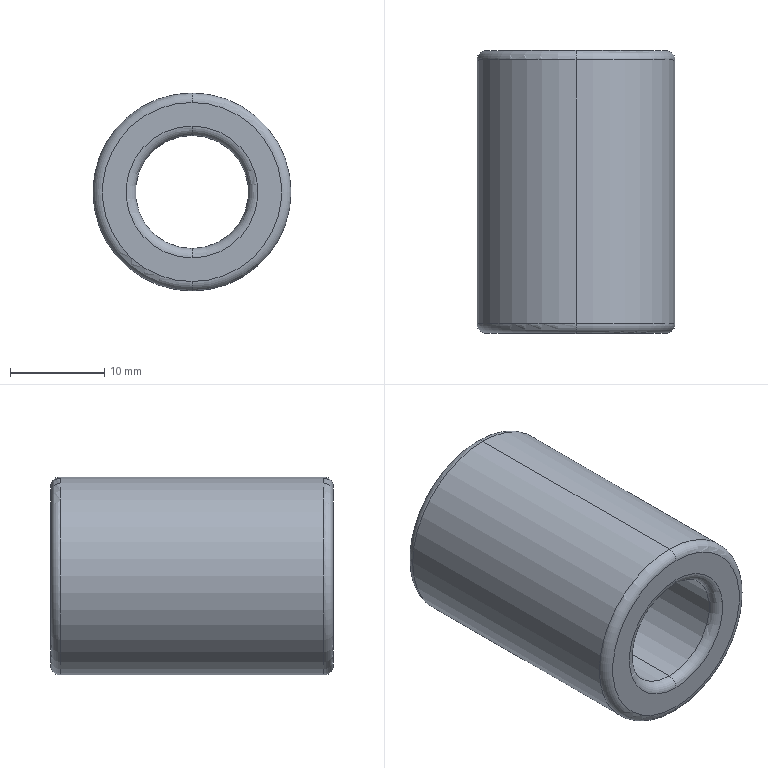Part | SolidWorks | features Extrusion 1, Fillet 1 | 1 solid | 14 faces | box 21 x 30 x 21 mm | volume 6953 mm3 | torus 8 | cylinder 4 | plane 2 | commonest cylinder face diameters 12 x2 21 x2
STEP:
#1=CARTESIAN_POINT('',(0.,29.,-10.5));
#2=VERTEX_POINT('',#1);
#3=CARTESIAN_POINT('',(0.,29.,10.5));
#4=VERTEX_POINT('',#3);
#5=CARTESIAN_POINT('',(0.,29.,0.));
#6=DIRECTION('',(0.,-1.,0.));
#7=DIRECTION('',(0.,0.,1.));
#8=AXIS2_PLACEMENT_3D('',#5,#6,#7);
#9=CIRCLE('',#8,10.5);
#10=EDGE_CURVE('',#2,#4,#9,.T.);
#11=ORIENTED_EDGE('',*,*,#10,.F.);
#12=CARTESIAN_POINT('',(0.,30.,-9.5));
#13=VERTEX_POINT('',#12);
#14=CARTESIAN_POINT('',(0.,29.,-9.5));
#15=DIRECTION('',(1.,0.,0.));
#16=DIRECTION('',(0.,0.,-1.));
#17=AXIS2_PLACEMENT_3D('',#14,#15,#16);
#18=CIRCLE('',#17,1.);
#19=EDGE_CURVE('',#2,#13,#18,.T.);
#20=ORIENTED_EDGE('',*,*,#19,.T.);
#21=CARTESIAN_POINT('',(0.,30.,9.5));
#22=VERTEX_POINT('',#21);
#23=CARTESIAN_POINT('',(0.,30.,0.));
#24=DIRECTION('',(0.,1.,0.));
#25=DIRECTION('',(0.,0.,1.));
#26=AXIS2_PLACEMENT_3D('',#23,#24,#25);
#27=CIRCLE('',#26,9.5);
#28=EDGE_CURVE('',#22,#13,#27,.T.);
#29=ORIENTED_EDGE('',*,*,#28,.F.);
#30=CARTESIAN_POINT('',(0.,29.,9.5));
#31=DIRECTION('',(-1.,0.,0.));
#32=DIRECTION('',(0.,0.,1.));
#33=AXIS2_PLACEMENT_3D('',#30,#31,#32);
#34=CIRCLE('',#33,1.);
#35=EDGE_CURVE('',#4,#22,#34,.T.);
#36=ORIENTED_EDGE('',*,*,#35,.F.);
#37=EDGE_LOOP('',(#11,#20,#29,#36));
#38=FACE_OUTER_BOUND('',#37,.T.);
#39=CARTESIAN_POINT('',(0.,29.,0.));
#40=DIRECTION('',(0.,1.,0.));
#41=DIRECTION('',(0.,0.,1.));
#42=AXIS2_PLACEMENT_3D('',#39,#40,#41);
#43=TOROIDAL_SURFACE('',#42,9.5,1.);
#44=ADVANCED_FACE('',(#38),#43,.T.);
#45=CARTESIAN_POINT('',(0.,0.,-9.5));
#46=VERTEX_POINT('',#45);
#47=CARTESIAN_POINT('',(0.,0.,9.5));
#48=VERTEX_POINT('',#47);
#49=CARTESIAN_POINT('',(0.,0.,0.));
#50=DIRECTION('',(0.,-1.,0.));
#51=DIRECTION('',(0.,0.,1.));
#52=AXIS2_PLACEMENT_3D('',#49,#50,#51);
#53=CIRCLE('',#52,9.5);
#54=EDGE_CURVE('',#46,#48,#53,.T.);
#55=ORIENTED_EDGE('',*,*,#54,.F.);
#56=CARTESIAN_POINT('',(0.,1.,-10.5));
#57=VERTEX_POINT('',#56);
#58=CARTESIAN_POINT('',(0.,1.,-9.5));
#59=DIRECTION('',(1.,0.,0.));
#60=DIRECTION('',(0.,0.,-1.));
#61=AXIS2_PLACEMENT_3D('',#58,#59,#60);
#62=CIRCLE('',#61,1.);
#63=EDGE_CURVE('',#46,#57,#62,.T.);
#64=ORIENTED_EDGE('',*,*,#63,.T.);
#65=CARTESIAN_POINT('',(0.,1.,10.5));
#66=VERTEX_POINT('',#65);
#67=CARTESIAN_POINT('',(0.,1.,0.));
#68=DIRECTION('',(0.,1.,0.));
#69=DIRECTION('',(0.,0.,1.));
#70=AXIS2_PLACEMENT_3D('',#67,#68,#69);
#71=CIRCLE('',#70,10.5);
#72=EDGE_CURVE('',#66,#57,#71,.T.);
#73=ORIENTED_EDGE('',*,*,#72,.F.);
#74=CARTESIAN_POINT('',(0.,1.,9.5));
#75=DIRECTION('',(-1.,0.,0.));
#76=DIRECTION('',(0.,0.,1.));
#77=AXIS2_PLACEMENT_3D('',#74,#75,#76);
#78=CIRCLE('',#77,1.);
#79=EDGE_CURVE('',#48,#66,#78,.T.);
#80=ORIENTED_EDGE('',*,*,#79,.F.);
#81=EDGE_LOOP('',(#55,#64,#73,#80));
#82=FACE_OUTER_BOUND('',#81,.T.);
#83=CARTESIAN_POINT('',(0.,1.,0.));
#84=DIRECTION('',(0.,1.,0.));
#85=DIRECTION('',(0.,0.,1.));
#86=AXIS2_PLACEMENT_3D('',#83,#84,#85);
#87=TOROIDAL_SURFACE('',#86,9.5,1.);
#88=ADVANCED_FACE('',(#82),#87,.T.);
#89=CARTESIAN_POINT('',(0.,30.,-7.));
#90=VERTEX_POINT('',#89);
#91=CARTESIAN_POINT('',(0.,30.,7.));
#92=VERTEX_POINT('',#91);
#93=CARTESIAN_POINT('',(0.,30.,0.));
#94=DIRECTION('',(0.,-1.,0.));
#95=DIRECTION('',(0.,0.,1.));
#96=AXIS2_PLACEMENT_3D('',#93,#94,#95);
#97=CIRCLE('',#96,7.);
#98=EDGE_CURVE('',#90,#92,#97,.T.);
#99=ORIENTED_EDGE('',*,*,#98,.F.);
#100=CARTESIAN_POINT('',(0.,29.,-6.));
#101=VERTEX_POINT('',#100);
#102=CARTESIAN_POINT('',(0.,29.,-7.));
#103=DIRECTION('',(1.,0.,0.));
#104=DIRECTION('',(0.,0.,-1.));
#105=AXIS2_PLACEMENT_3D('',#102,#103,#104);
#106=CIRCLE('',#105,1.);
#107=EDGE_CURVE('',#90,#101,#106,.T.);
#108=ORIENTED_EDGE('',*,*,#107,.T.);
#109=CARTESIAN_POINT('',(0.,29.,6.));
#110=VERTEX_POINT('',#109);
#111=CARTESIAN_POINT('',(0.,29.,0.));
#112=DIRECTION('',(0.,1.,0.));
#113=DIRECTION('',(0.,0.,1.));
#114=AXIS2_PLACEMENT_3D('',#111,#112,#113);
#115=CIRCLE('',#114,6.);
#116=EDGE_CURVE('',#110,#101,#115,.T.);
#117=ORIENTED_EDGE('',*,*,#116,.F.);
#118=CARTESIAN_POINT('',(0.,29.,7.));
#119=DIRECTION('',(-1.,0.,0.));
#120=DIRECTION('',(0.,0.,1.));
#121=AXIS2_PLACEMENT_3D('',#118,#119,#120);
#122=CIRCLE('',#121,1.);
#123=EDGE_CURVE('',#92,#110,#122,.T.);
#124=ORIENTED_EDGE('',*,*,#123,.F.);
#125=EDGE_LOOP('',(#99,#108,#117,#124));
#126=FACE_OUTER_BOUND('',#125,.T.);
#127=CARTESIAN_POINT('',(0.,29.,0.));
#128=DIRECTION('',(0.,1.,0.));
#129=DIRECTION('',(0.,0.,1.));
#130=AXIS2_PLACEMENT_3D('',#127,#128,#129);
#131=TOROIDAL_SURFACE('',#130,7.,1.);
#132=ADVANCED_FACE('',(#126),#131,.T.);
#133=CARTESIAN_POINT('',(0.,1.,-6.));
#134=VERTEX_POINT('',#133);
#135=CARTESIAN_POINT('',(0.,1.,6.));
#136=VERTEX_POINT('',#135);
#137=CARTESIAN_POINT('',(0.,1.,0.));
#138=DIRECTION('',(0.,-1.,0.));
#139=DIRECTION('',(0.,0.,1.));
#140=AXIS2_PLACEMENT_3D('',#137,#138,#139);
#141=CIRCLE('',#140,6.);
#142=EDGE_CURVE('',#134,#136,#141,.T.);
#143=ORIENTED_EDGE('',*,*,#142,.F.);
#144=CARTESIAN_POINT('',(0.,0.,-7.));
#145=VERTEX_POINT('',#144);
#146=CARTESIAN_POINT('',(0.,1.,-7.));
#147=DIRECTION('',(1.,0.,0.));
#148=DIRECTION('',(0.,0.,-1.));
#149=AXIS2_PLACEMENT_3D('',#146,#147,#148);
#150=CIRCLE('',#149,1.);
#151=EDGE_CURVE('',#134,#145,#150,.T.);
#152=ORIENTED_EDGE('',*,*,#151,.T.);
#153=CARTESIAN_POINT('',(0.,0.,7.));
#154=VERTEX_POINT('',#153);
#155=CARTESIAN_POINT('',(0.,0.,0.));
#156=DIRECTION('',(0.,1.,0.));
#157=DIRECTION('',(0.,0.,1.));
#158=AXIS2_PLACEMENT_3D('',#155,#156,#157);
#159=CIRCLE('',#158,7.);
#160=EDGE_CURVE('',#154,#145,#159,.T.);
#161=ORIENTED_EDGE('',*,*,#160,.F.);
#162=CARTESIAN_POINT('',(0.,1.,7.));
#163=DIRECTION('',(-1.,0.,0.));
#164=DIRECTION('',(0.,0.,1.));
#165=AXIS2_PLACEMENT_3D('',#162,#163,#164);
#166=CIRCLE('',#165,1.);
#167=EDGE_CURVE('',#136,#154,#166,.T.);
#168=ORIENTED_EDGE('',*,*,#167,.F.);
#169=EDGE_LOOP('',(#143,#152,#161,#168));
#170=FACE_OUTER_BOUND('',#169,.T.);
#171=CARTESIAN_POINT('',(0.,1.,0.));
#172=DIRECTION('',(0.,1.,0.));
#173=DIRECTION('',(0.,0.,1.));
#174=AXIS2_PLACEMENT_3D('',#171,#172,#173);
#175=TOROIDAL_SURFACE('',#174,7.,1.);
#176=ADVANCED_FACE('',(#170),#175,.T.);
#177=CARTESIAN_POINT('',(0.,29.,0.));
#178=DIRECTION('',(0.,1.,0.));
#179=DIRECTION('',(0.,0.,1.));
#180=AXIS2_PLACEMENT_3D('',#177,#178,#179);
#181=CIRCLE('',#180,6.);
#182=EDGE_CURVE('',#101,#110,#181,.T.);
#183=ORIENTED_EDGE('',*,*,#182,.T.);
#184=CARTESIAN_POINT('',(0.,30.,6.));
#185=DIRECTION('',(0.,-1.,0.));
#186=VECTOR('',#185,1000.);
#187=LINE('',#184,#186);
#188=EDGE_CURVE('',#110,#136,#187,.T.);
#189=ORIENTED_EDGE('',*,*,#188,.T.);
#190=CARTESIAN_POINT('',(0.,1.,0.));
#191=DIRECTION('',(0.,-1.,0.));
#192=DIRECTION('',(0.,0.,1.));
#193=AXIS2_PLACEMENT_3D('',#190,#191,#192);
#194=CIRCLE('',#193,6.);
#195=EDGE_CURVE('',#136,#134,#194,.T.);
#196=ORIENTED_EDGE('',*,*,#195,.T.);
#197=CARTESIAN_POINT('',(0.,30.,-6.));
#198=DIRECTION('',(0.,-1.,0.));
#199=VECTOR('',#198,1000.);
#200=LINE('',#197,#199);
#201=EDGE_CURVE('',#101,#134,#200,.T.);
#202=ORIENTED_EDGE('',*,*,#201,.F.);
#203=EDGE_LOOP('',(#183,#189,#196,#202));
#204=FACE_OUTER_BOUND('',#203,.T.);
#205=CARTESIAN_POINT('',(0.,30.,0.));
#206=DIRECTION('',(0.,-1.,0.));
#207=DIRECTION('',(0.,0.,-1.));
#208=AXIS2_PLACEMENT_3D('',#205,#206,#207);
#209=CYLINDRICAL_SURFACE('',#208,6.);
#210=ADVANCED_FACE('',(#204),#209,.F.);
#211=ORIENTED_EDGE('',*,*,#10,.T.);
#212=CARTESIAN_POINT('',(0.,30.,10.5));
#213=DIRECTION('',(0.,-1.,0.));
#214=VECTOR('',#213,1000.);
#215=LINE('',#212,#214);
#216=EDGE_CURVE('',#4,#66,#215,.T.);
#217=ORIENTED_EDGE('',*,*,#216,.T.);
#218=ORIENTED_EDGE('',*,*,#72,.T.);
#219=CARTESIAN_POINT('',(0.,30.,-10.5));
#220=DIRECTION('',(0.,-1.,0.));
#221=VECTOR('',#220,1000.);
#222=LINE('',#219,#221);
#223=EDGE_CURVE('',#2,#57,#222,.T.);
#224=ORIENTED_EDGE('',*,*,#223,.F.);
#225=EDGE_LOOP('',(#211,#217,#218,#224));
#226=FACE_OUTER_BOUND('',#225,.T.);
#227=CARTESIAN_POINT('',(0.,30.,0.));
#228=DIRECTION('',(0.,-1.,0.));
#229=DIRECTION('',(0.,0.,-1.));
#230=AXIS2_PLACEMENT_3D('',#227,#228,#229);
#231=CYLINDRICAL_SURFACE('',#230,10.5);
#232=ADVANCED_FACE('',(#226),#231,.T.);
#233=CARTESIAN_POINT('',(0.,30.,0.));
#234=DIRECTION('',(0.,-1.,0.));
#235=DIRECTION('',(0.,0.,1.));
#236=AXIS2_PLACEMENT_3D('',#233,#234,#235);
#237=CIRCLE('',#236,7.);
#238=EDGE_CURVE('',#92,#90,#237,.T.);
#239=ORIENTED_EDGE('',*,*,#238,.T.);
#240=ORIENTED_EDGE('',*,*,#98,.T.);
#241=EDGE_LOOP('',(#239,#240));
#242=FACE_BOUND('',#241,.T.);
#243=ORIENTED_EDGE('',*,*,#28,.T.);
#244=CARTESIAN_POINT('',(0.,30.,0.));
#245=DIRECTION('',(0.,1.,0.));
#246=DIRECTION('',(0.,0.,1.));
#247=AXIS2_PLACEMENT_3D('',#244,#245,#246);
#248=CIRCLE('',#247,9.5);
#249=EDGE_CURVE('',#13,#22,#248,.T.);
#250=ORIENTED_EDGE('',*,*,#249,.T.);
#251=EDGE_LOOP('',(#243,#250));
#252=FACE_OUTER_BOUND('',#251,.T.);
#253=CARTESIAN_POINT('',(0.,30.,0.));
#254=DIRECTION('',(0.,1.,0.));
#255=DIRECTION('',(0.,0.,1.));
#256=AXIS2_PLACEMENT_3D('',#253,#254,#255);
#257=PLANE('',#256);
#258=ADVANCED_FACE('',(#242,#252),#257,.T.);
#259=ORIENTED_EDGE('',*,*,#160,.T.);
#260=CARTESIAN_POINT('',(0.,0.,0.));
#261=DIRECTION('',(0.,1.,0.));
#262=DIRECTION('',(0.,0.,1.));
#263=AXIS2_PLACEMENT_3D('',#260,#261,#262);
#264=CIRCLE('',#263,7.);
#265=EDGE_CURVE('',#145,#154,#264,.T.);
#266=ORIENTED_EDGE('',*,*,#265,.T.);
#267=EDGE_LOOP('',(#259,#266));
#268=FACE_BOUND('',#267,.T.);
#269=CARTESIAN_POINT('',(0.,0.,0.));
#270=DIRECTION('',(0.,-1.,0.));
#271=DIRECTION('',(0.,0.,1.));
#272=AXIS2_PLACEMENT_3D('',#269,#270,#271);
#273=CIRCLE('',#272,9.5);
#274=EDGE_CURVE('',#48,#46,#273,.T.);
#275=ORIENTED_EDGE('',*,*,#274,.T.);
#276=ORIENTED_EDGE('',*,*,#54,.T.);
#277=EDGE_LOOP('',(#275,#276));
#278=FACE_OUTER_BOUND('',#277,.T.);
#279=CARTESIAN_POINT('',(0.,0.,0.));
#280=DIRECTION('',(0.,1.,0.));
#281=DIRECTION('',(0.,0.,1.));
#282=AXIS2_PLACEMENT_3D('',#279,#280,#281);
#283=PLANE('',#282);
#284=ADVANCED_FACE('',(#268,#278),#283,.F.);
#285=ORIENTED_EDGE('',*,*,#216,.F.);
#286=CARTESIAN_POINT('',(0.,29.,0.));
#287=DIRECTION('',(0.,-1.,0.));
#288=DIRECTION('',(0.,0.,1.));
#289=AXIS2_PLACEMENT_3D('',#286,#287,#288);
#290=CIRCLE('',#289,10.5);
#291=EDGE_CURVE('',#4,#2,#290,.T.);
#292=ORIENTED_EDGE('',*,*,#291,.T.);
#293=ORIENTED_EDGE('',*,*,#223,.T.);
#294=CARTESIAN_POINT('',(0.,1.,0.));
#295=DIRECTION('',(0.,1.,0.));
#296=DIRECTION('',(0.,0.,1.));
#297=AXIS2_PLACEMENT_3D('',#294,#295,#296);
#298=CIRCLE('',#297,10.5);
#299=EDGE_CURVE('',#57,#66,#298,.T.);
#300=ORIENTED_EDGE('',*,*,#299,.T.);
#301=EDGE_LOOP('',(#285,#292,#293,#300));
#302=FACE_OUTER_BOUND('',#301,.T.);
#303=CARTESIAN_POINT('',(0.,30.,0.));
#304=DIRECTION('',(0.,-1.,0.));
#305=DIRECTION('',(0.,0.,-1.));
#306=AXIS2_PLACEMENT_3D('',#303,#304,#305);
#307=CYLINDRICAL_SURFACE('',#306,10.5);
#308=ADVANCED_FACE('',(#302),#307,.T.);
#309=ORIENTED_EDGE('',*,*,#188,.F.);
#310=ORIENTED_EDGE('',*,*,#116,.T.);
#311=ORIENTED_EDGE('',*,*,#201,.T.);
#312=ORIENTED_EDGE('',*,*,#142,.T.);
#313=EDGE_LOOP('',(#309,#310,#311,#312));
#314=FACE_OUTER_BOUND('',#313,.T.);
#315=CARTESIAN_POINT('',(0.,30.,0.));
#316=DIRECTION('',(0.,-1.,0.));
#317=DIRECTION('',(0.,0.,-1.));
#318=AXIS2_PLACEMENT_3D('',#315,#316,#317);
#319=CYLINDRICAL_SURFACE('',#318,6.);
#320=ADVANCED_FACE('',(#314),#319,.F.);
#321=ORIENTED_EDGE('',*,*,#151,.F.);
#322=ORIENTED_EDGE('',*,*,#195,.F.);
#323=ORIENTED_EDGE('',*,*,#167,.T.);
#324=ORIENTED_EDGE('',*,*,#265,.F.);
#325=EDGE_LOOP('',(#321,#322,#323,#324));
#326=FACE_OUTER_BOUND('',#325,.T.);
#327=CARTESIAN_POINT('',(0.,1.,0.));
#328=DIRECTION('',(0.,1.,0.));
#329=DIRECTION('',(0.,0.,1.));
#330=AXIS2_PLACEMENT_3D('',#327,#328,#329);
#331=TOROIDAL_SURFACE('',#330,7.,1.);
#332=ADVANCED_FACE('',(#326),#331,.T.);
#333=ORIENTED_EDGE('',*,*,#107,.F.);
#334=ORIENTED_EDGE('',*,*,#238,.F.);
#335=ORIENTED_EDGE('',*,*,#123,.T.);
#336=ORIENTED_EDGE('',*,*,#182,.F.);
#337=EDGE_LOOP('',(#333,#334,#335,#336));
#338=FACE_OUTER_BOUND('',#337,.T.);
#339=CARTESIAN_POINT('',(0.,29.,0.));
#340=DIRECTION('',(0.,1.,0.));
#341=DIRECTION('',(0.,0.,1.));
#342=AXIS2_PLACEMENT_3D('',#339,#340,#341);
#343=TOROIDAL_SURFACE('',#342,7.,1.);
#344=ADVANCED_FACE('',(#338),#343,.T.);
#345=ORIENTED_EDGE('',*,*,#63,.F.);
#346=ORIENTED_EDGE('',*,*,#274,.F.);
#347=ORIENTED_EDGE('',*,*,#79,.T.);
#348=ORIENTED_EDGE('',*,*,#299,.F.);
#349=EDGE_LOOP('',(#345,#346,#347,#348));
#350=FACE_OUTER_BOUND('',#349,.T.);
#351=CARTESIAN_POINT('',(0.,1.,0.));
#352=DIRECTION('',(0.,1.,0.));
#353=DIRECTION('',(0.,0.,1.));
#354=AXIS2_PLACEMENT_3D('',#351,#352,#353);
#355=TOROIDAL_SURFACE('',#354,9.5,1.);
#356=ADVANCED_FACE('',(#350),#355,.T.);
#357=ORIENTED_EDGE('',*,*,#19,.F.);
#358=ORIENTED_EDGE('',*,*,#291,.F.);
#359=ORIENTED_EDGE('',*,*,#35,.T.);
#360=ORIENTED_EDGE('',*,*,#249,.F.);
#361=EDGE_LOOP('',(#357,#358,#359,#360));
#362=FACE_OUTER_BOUND('',#361,.T.);
#363=CARTESIAN_POINT('',(0.,29.,0.));
#364=DIRECTION('',(0.,1.,0.));
#365=DIRECTION('',(0.,0.,1.));
#366=AXIS2_PLACEMENT_3D('',#363,#364,#365);
#367=TOROIDAL_SURFACE('',#366,9.5,1.);
#368=ADVANCED_FACE('',(#362),#367,.T.);
#369=CLOSED_SHELL('',(#44,#88,#132,#176,#210,#232,#258,#284,#308,#320,#332,#344,#356,#368));
#370=MANIFOLD_SOLID_BREP('',#369);
#371=CARTESIAN_POINT('',(0.,0.,0.));
#372=DIRECTION('',(0.,0.,1.));
#373=DIRECTION('',(1.,0.,0.));
#374=AXIS2_PLACEMENT_3D('',#371,#372,#373);
#375=(LENGTH_UNIT()NAMED_UNIT(*)SI_UNIT(.MILLI.,.METRE.));
#376=UNCERTAINTY_MEASURE_WITH_UNIT(LENGTH_MEASURE(0.00001),#375,'','');
#377=(NAMED_UNIT(*)PLANE_ANGLE_UNIT()SI_UNIT($,.RADIAN.));
#378=(NAMED_UNIT(*)SI_UNIT($,.STERADIAN.)SOLID_ANGLE_UNIT());
#379=(GEOMETRIC_REPRESENTATION_CONTEXT(3)GLOBAL_UNCERTAINTY_ASSIGNED_CONTEXT((#376))GLOBAL_UNIT_ASSIGNED_CONTEXT((#375,#377,#378))REPRESENTATION_CONTEXT('',''));
#380=ADVANCED_BREP_SHAPE_REPRESENTATION('',(#370,#374),#379);